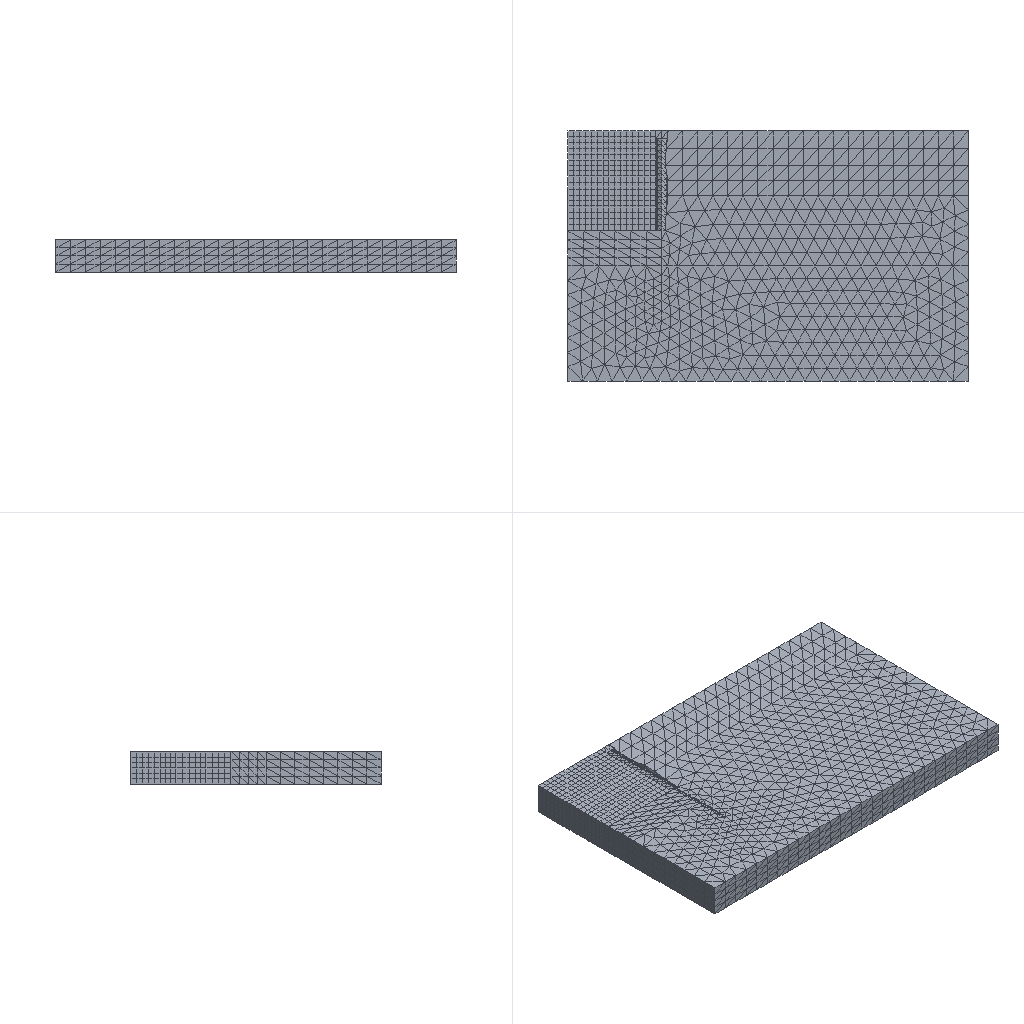Simulation study | abaqus
Set-up summary:
category,name,step,type,value,unit,region
solver,abaqus
solver,version,,,Abaqus/Standard 2020
units,not stated in the deck,,not stated
analysis,deck,,static,static
load_step,Step-delete-all,Step-delete-all,static
load_step,Step-add-zhuang,Step-add-zhuang,static
load_step,Step-geo-final,Step-geo-final,geostatic
load_step,Step-dig-lay1,Step-dig-lay1,static
load_step,Step-add-maosuo1,Step-add-maosuo1,static
load_step,Step-dig-lay2,Step-dig-lay2,static
load_step,Step-add-maosuo2,Step-add-maosuo2,static
load_step,Step-dig-lay3,Step-dig-lay3,static
load_step,requested,,,8
mesh,nodes,,,14615
mesh,elements,,,20579
element_type,C3D4,,solid,13823
element_type,T3D2,,truss,20
element_type,C3D8R,,solid,6736
load,load commands in deck,,count,9
bc,support commands in deck,,count,28
material,LAY-1,,in results
material,LAY-2,,in results
material,LAY-3,,in results
material,LAY-4,,in results
material,MAOSUO,,in results
material,STEEL,,in results
material,ZHUANG-CEMENT,,in results
material,ZHUANG-HUBI,,in results
check,setup vs results,,match,"per instance, exact: element labels, types and connectivity; labels of the nodes the elements use; coordinates of those nodes at SINGLE_PRECISION in 4 of 7 instance(s)"
Abaqus input file, long lists of numbers shortened:
*Heading
** Job name: Job-1 Model name: Model-1
** Generated by: Abaqus/CAE 2020
*Preprint, echo=NO, model=NO, history=NO, contact=NO
**
** PARTS
**
*Part, name=Part-2
*Node
      1,        -250.,      -10000.,        1850.
      2,  -355.051,      -10000.,        1600.
** (2613 more lines like these left out)
*Element, type=C3D4
   1, 1661, 1662,  800,  799
   2, 1661, 1663, 1664, 1665
** (11001 more lines like these left out)
*Nset, nset=Set-1
   47,   48,   49,   50,   51,   52,   63,   64,   65,   66,  254,  255,  256,  258,  259,  260
  261,  262,  263,  264,  265,  266,  267,  268,  269,  270,  271,  272,  273,  274,  275,  276
** (21 more lines like these left out)
*Elset, elset=Set-1, generate
  9778,  11003,      1
*Nset, nset=Set-2
   20,   21,   22,   23,   26,   27,   47,   48,   49,   50,   51,   52,   83,   87,   88,   89
   90,   91,   92,   93,   94,   95,   96,   97,   98,   99,  100,  101,  102,  103,  104,  105
** (20 more lines like these left out)
*Elset, elset=Set-2, generate
 3019,  4197,     1
*Nset, nset=Set-3
    1,    2,    3,    4,    5,    6,    7,    8,    9,   10,   11,   12,   13,   14,   15,   16
   17,   18,   19,   20,   21,   22,   23,   24,   25,   26,   27,   28,   29,   30,   31,   32
** (51 more lines like these left out)
*Elset, elset=Set-3, generate
    1,  3018,     1
*Nset, nset=Set-4
   33,   34,   35,   37,   38,   40,   41,   42,   43,   46,   53,   54,   55,   56,   57,   58
   59,   60,   61,   62,  141,  142,  143,  144,  145,  146,  147,  148,  149,  150,  151,  152
** (85 more lines like these left out)
*Elset, elset=Set-4, generate
 4198,  9777,     1
** Section: lay3
*Solid Section, elset=Set-3, material=lay-3
,
** Section: lay-2
*Solid Section, elset=Set-2, material=lay-2
,
** Section: lay4
*Solid Section, elset=Set-4, material=lay-4
,
** Section: lay1
*Solid Section, elset=Set-1, material=lay-1
,
*End Part
**
*Part, name=Part-4
*Node
      1,  -198.585,  -2785.345,   3474.874
      2,  -198.585,  -11785.345,   3474.874
** (800 more lines like these left out)
*Element, type=C3D4
  1, 313, 333, 115, 116
  2, 275,  37, 625, 258
** (2818 more lines like these left out)
*Nset, nset=Set-4
   1,   2,   5,   6,   7,   8,   9,  12,  13,  14,  15,  16,  17,  26,  28,  29
  31,  32,  33,  34,  35,  36,  37,  38,  39,  40,  41,  42,  43,  44,  45,  60
** (39 more lines like these left out)
*Elset, elset=Set-4
  630,  631,  632,  633,  634,  635,  636,  637,  638,  639,  640,  641,  642,  643,  644,  645
  646,  647,  648,  649,  650,  651,  652,  653,  654,  655,  656,  657,  658,  659,  660,  661
** (127 more lines like these left out)
*Nset, nset=Set-5
   1,   2,   3,   4,   5,   6,   7,   8,   9,  10,  11,  12,  34,  35,  36,  37
  38,  39,  40,  41,  42,  43,  44,  45,  46,  47,  48,  49,  50,  51,  52,  53
** (11 more lines like these left out)
*Elset, elset=Set-5, generate
   1,  629,    1
*Nset, nset=Set-6
  13,  14,  15,  18,  19,  20,  21,  22,  23,  24,  25,  26,  27,  28,  29,  30
 118, 119, 120, 121, 122, 183, 184, 185, 186, 187, 188, 189, 190, 191, 192, 193
** (2 more lines like these left out)
*Elset, elset=Set-6, generate
 1645,  1779,     1
** Section: zhuang-cement
*Solid Section, elset=Set-5, material=zhuang-cement
,
** Section: zhuang-hubi
*Solid Section, elset=Set-4, material=zhuang-hubi
,
** Section: zhuang-hubi
*Solid Section, elset=Set-6, material=zhuang-hubi
,
*End Part
**
*Part, name=digit
*Node
      1,        8800.,       -7500.,           0.
      2,        8800.,       -7500.,        3200.
** (2014 more lines like these left out)
*Element, type=C3D8R
  1,   84,  415, 1177,  331,    1,   25,  301,   40
  2,  415,  416, 1178, 1177,   25,   26,  302,  301
** (1528 more lines like these left out)
*Nset, nset=Set-1
   11,   12,   14,   15,   21,   22,   23,   24,  119,  120,  121,  122,  123,  131,  132,  133
  134,  135,  137,  138,  139,  140,  141,  142,  143,  144,  145,  146,  147,  148,  149,  150
** (47 more lines like these left out)
*Elset, elset=Set-1, generate
  991,  1530,     1
*Nset, nset=Set-2
    9,   10,   11,   12,   13,   14,   15,   16,   17,   18,   19,   20,  113,  114,  115,  116
  117,  118,  119,  120,  121,  122,  123,  124,  125,  126,  127,  128,  129,  130,  131,  132
** (40 more lines like these left out)
*Elset, elset=Set-2
 361, 362, 363, 364, 365, 366, 367, 368, 369, 370, 371, 372, 373, 374, 375, 376
 377, 378, 379, 380, 381, 382, 383, 384, 385, 386, 387, 388, 389, 390, 391, 392
** (27 more lines like these left out)
*Nset, nset=Set-3
    1,    2,    3,    4,    5,    6,    7,    8,   17,   18,   19,   20,   25,   26,   27,   28
   29,   30,   31,   32,   33,   34,   35,   36,   37,   38,   39,   40,   41,   42,   43,   44
** (47 more lines like these left out)
*Elset, elset=Set-3
   1,   2,   3,   4,   5,   6,   7,   8,   9,  10,  11,  12,  13,  14,  15,  16
  17,  18,  19,  20,  21,  22,  23,  24,  25,  26,  27,  28,  29,  30,  31,  32
** (32 more lines like these left out)
*Nset, nset=dig
    9,   10,   11,   12,   13,   14,   15,   16,   21,   22,   23,   24,  113,  114,  115,  116
  117,  118,  119,  120,  121,  122,  123,  124,  125,  126,  127,  128,  129,  130,  131,  132
** (61 more lines like these left out)
*Elset, elset=dig
  361,  362,  363,  364,  365,  366,  367,  368,  369,  370,  371,  372,  373,  374,  375,  376
  377,  378,  379,  380,  381,  382,  383,  384,  385,  386,  387,  388,  389,  390,  391,  392
** (43 more lines like these left out)
*Nset, nset=dig2
    1,    2,    5,    8,    9,   10,   13,   16,   17,   18,   19,   20,   25,   26,   27,   28
   29,   41,   42,   43,   44,   45,   71,   72,   73,   74,   75,   76,   77,   78,   79,   80
** (40 more lines like these left out)
*Elset, elset=dig2, generate
 541,  990,    1
*Nset, nset=dig3
    1,    2,    3,    4,    5,    6,    7,    8,   25,   26,   27,   28,   29,   30,   31,   32
   33,   34,   35,   36,   37,   38,   39,   40,   41,   42,   43,   44,   45,   46,   47,   48
** (33 more lines like these left out)
*Elset, elset=dig3, generate
   1,  360,    1
*Nset, nset=Set-9
    9,   10,   11,   12,   13,   14,   15,   16,   21,   22,   23,   24,  113,  114,  115,  116
  117,  118,  119,  120,  121,  122,  123,  124,  125,  126,  127,  128,  129,  130,  131,  132
** (61 more lines like these left out)
*Elset, elset=Set-9
  361,  362,  363,  364,  365,  366,  367,  368,  369,  370,  371,  372,  373,  374,  375,  376
  377,  378,  379,  380,  381,  382,  383,  384,  385,  386,  387,  388,  389,  390,  391,  392
** (43 more lines like these left out)
*Nset, nset=Set-10
    1,    2,    5,    8,    9,   10,   13,   16,   17,   18,   19,   20,   25,   26,   27,   28
   29,   41,   42,   43,   44,   45,   71,   72,   73,   74,   75,   76,   77,   78,   79,   80
** (40 more lines like these left out)
*Elset, elset=Set-10, generate
 541,  990,    1
*Nset, nset=Set-11
    1,    2,    3,    4,    5,    6,    7,    8,   25,   26,   27,   28,   29,   30,   31,   32
   33,   34,   35,   36,   37,   38,   39,   40,   41,   42,   43,   44,   45,   46,   47,   48
** (33 more lines like these left out)
*Elset, elset=Set-11, generate
   1,  360,    1
*Nset, nset=Set-12
   11,   12,   14,   15,   21,   22,   23,   24,  119,  120,  121,  122,  123,  131,  132,  133
  134,  135,  137,  138,  139,  140,  141,  142,  143,  144,  145,  146,  147,  148,  149,  150
** (47 more lines like these left out)
*Elset, elset=Set-12, generate
  991,  1530,     1
*Nset, nset=Set-13
    9,   10,   11,   12,   13,   14,   15,   16,   17,   18,   19,   20,  113,  114,  115,  116
  117,  118,  119,  120,  121,  122,  123,  124,  125,  126,  127,  128,  129,  130,  131,  132
** (40 more lines like these left out)
*Elset, elset=Set-13
 361, 362, 363, 364, 365, 366, 367, 368, 369, 370, 371, 372, 373, 374, 375, 376
 377, 378, 379, 380, 381, 382, 383, 384, 385, 386, 387, 388, 389, 390, 391, 392
** (27 more lines like these left out)
*Nset, nset=Set-14
    1,    2,    3,    4,    5,    6,    7,    8,   17,   18,   19,   20,   25,   26,   27,   28
   29,   30,   31,   32,   33,   34,   35,   36,   37,   38,   39,   40,   41,   42,   43,   44
** (47 more lines like these left out)
*Elset, elset=Set-14
   1,   2,   3,   4,   5,   6,   7,   8,   9,  10,  11,  12,  13,  14,  15,  16
  17,  18,  19,  20,  21,  22,  23,  24,  25,  26,  27,  28,  29,  30,  31,  32
** (32 more lines like these left out)
** Section: lay3
*Solid Section, elset=Set-14, material=lay-3
,
** Section: lay-2
*Solid Section, elset=Set-13, material=lay-2
,
** Section: lay1
*Solid Section, elset=Set-12, material=lay-1
,
*End Part
**
*Part, name=maosuo-d27
*Node
      1,           0.,           0.,           0.
      2,   1556.389,  -1089.795,           0.
** (9 more lines like these left out)
*Element, type=T3D2
 1,  1,  2
 2,  2,  3
** (8 more lines like these left out)
*Nset, nset=Set-1, generate
  1,  11,   1
*Elset, elset=Set-1, generate
  1,  10,   1
** Section: maosuo-d27
*Solid Section, elset=Set-1, material=maosuo
572.,
*End Part
**
*Part, name=maosuo-d33
*Node
      1,           0.,           0.,           0.
      2,   1884.05,  -1319.226,           0.
** (9 more lines like these left out)
*Element, type=T3D2
 1,  1,  2
 2,  2,  3
** (8 more lines like these left out)
*Nset, nset=Set-1, generate
  1,  11,   1
*Elset, elset=Set-1, generate
  1,  10,   1
** Section: mosuo-d33
*Solid Section, elset=Set-1, material=maosuo
855.,
*End Part
**
*Part, name=work-5
*Node
      1,  -345.475,   11544.227,        3350.
      2,  -45.475,   11544.227,        3350.
** (4578 more lines like these left out)
*Element, type=C3D8R
  1,  239,  240, 1295, 1296,  339,  340, 1342, 1343
  2,  166, 1280, 1279,  165,  266, 1327, 1326,  265
** (2601 more lines like these left out)
*Nset, nset=Set-2, generate
    1,  4580,     1
*Elset, elset=Set-2, generate
    1,  2603,     1
*Nset, nset=work5-insert-down
   25,   26,   27,   28,   29,   30,   31,   32,   33,   34,   35,   36,   37,   38,   39,   40
   41,   42,   43,   44,   45,   46,   47,   48,   49,   50,   51,   52,   53,   54,   55,   56
** (172 more lines like these left out)
*Elset, elset=work5-insert-down, generate
  686,  2603,     1
*Nset, nset=w5-insert-up
    1,    2,    3,    4,    5,    6,    7,    8,    9,   10,   11,   12,   13,   14,   15,   16
   17,   18,   19,   20,   21,   22,   23,   24,   73,   74,   75,   76,   77,   78,   79,   80
** (24 more lines like these left out)
*Elset, elset=w5-insert-up, generate
   1,  137,    1
** Section: steel
*Solid Section, elset=Set-2, material=steel
,
*End Part
**
**
** ASSEMBLY
**
*Assembly, name=Assembly
**
*Instance, name=Part-2-1, part=Part-2
*End Instance
**
*Instance, name=work-5-2, part=work-5
       2600.,  -155.773,  1654.525
       2600.,  -155.773,  1654.525, 2600.707,  -155.773, 1653.818,         180.
*End Instance
**
*Instance, name=digit-1, part=digit
     -10000.,           0.,           0.
*End Instance
**
*Instance, name=Part-4-1, part=Part-4
      -3800.,  -714.655,  1868.082
      -3800.,  -714.655,  1868.082,       -3800., -713.655,  1868.082, 90.
*End Instance
**
*Instance, name=maosuo-d27-1, part=maosuo-d27
          0.,       -7000.,        2600.
*End Instance
**
*Instance, name=maosuo-d33-1, part=maosuo-d33
          0.,       -4000.,         600.
*End Instance
**
*Instance, name=work-5-1, part=work-5
      -3800., -155.773,  1545.475
      -3800., -155.773,  1545.475, -3799.293, -155.773, 1546.182,         180.
*End Instance
**
*Nset, nset=Set-3, instance=maosuo-d27-1, generate
  1,  11,   1
*Nset, nset=Set-3, instance=maosuo-d33-1, generate
  1,  11,   1
*Elset, elset=Set-3, instance=maosuo-d27-1, generate
  1,  10,   1
*Elset, elset=Set-3, instance=maosuo-d33-1, generate
  1,  10,   1
*Nset, nset=Set-4, instance=maosuo-d27-1, generate
  1,  11,   1
*Nset, nset=Set-4, instance=maosuo-d33-1, generate
  1,  11,   1
*Elset, elset=Set-4, instance=maosuo-d27-1, generate
  1,  10,   1
*Elset, elset=Set-4, instance=maosuo-d33-1, generate
  1,  10,   1
*Nset, nset=Set-7, instance=Part-2-1
   59,   60,   61,   62,  334,  335,  336,  351,  352,  353,  354,  355,  356,  357,  358,  359
  360,  361,  362,  363,  364,  365,  366,  367,  368,  369,  370,  371,  372,  373,  374,  375
** (7 more lines like these left out)
*Elset, elset=Set-7, instance=Part-2-1
 4241, 4282, 4399, 4468, 4559, 4637, 4778, 5047, 5050, 5090, 5092, 5094, 5098, 5100, 5213, 5425
 5574, 5599, 5677, 5757, 5792, 5802, 5857, 5866, 5912, 5920, 5933, 5943, 5945, 5948, 5957, 6032
** (12 more lines like these left out)
*Nset, nset=Set-8, instance=Part-2-1
   26,   27,   34,   42,   43,   44,   45,   46,   47,   48,   59,   60,   61,   62,   63,   64
  106,  107,  108,  161,  162,  163,  164,  194,  195,  196,  197,  218,  219,  220,  226,  227
** (8 more lines like these left out)
*Elset, elset=Set-8, instance=Part-2-1
    65,    70,    86,    87,    88,   132,   137,   260,   350,   395,   401,   458,   474,   475,   566,   653
   880,  1001,  1120,  1123,  1180,  1181,  1210,  1329,  1339,  1509,  1510,  1511,  1515,  1567,  1571,  1628
** (13 more lines like these left out)
*Nset, nset=Set-9, instance=Part-2-1
    8,    9,   20,   23,   24,   25,   26,   27,   33,   34,   38,   42,   43,   44,   45,   46
   47,   48,   49,   50,   53,   58,   59,   60,   61,   62,   63,   64,   65,   66,   84,   85
** (64 more lines like these left out)
*Elset, elset=Set-9, instance=Part-2-1
    11,    16,    25,    49,    53,    58,    63,    67,    86,    89,   105,   107,   160,   162,   173,   186
   196,   210,   235,   241,   245,   248,   275,   280,   282,   295,   297,   324,   327,   335,   369,   382
** (118 more lines like these left out)
*Nset, nset=Set-15, instance=work-5-2, generate
    1,  4580,     1
*Nset, nset=Set-15, instance=Part-4-1, generate
   1,  802,    1
*Nset, nset=Set-15, instance=maosuo-d27-1, generate
  1,  11,   1
*Nset, nset=Set-15, instance=maosuo-d33-1, generate
  1,  11,   1
*Nset, nset=Set-15, instance=work-5-1, generate
    1,  4580,     1
*Elset, elset=Set-15, instance=work-5-2, generate
    1,  2603,     1
*Elset, elset=Set-15, instance=Part-4-1, generate
    1,  2820,     1
*Elset, elset=Set-15, instance=maosuo-d27-1, generate
  1,  10,   1
*Elset, elset=Set-15, instance=maosuo-d33-1, generate
  1,  10,   1
*Elset, elset=Set-15, instance=work-5-1, generate
    1,  2603,     1
*Nset, nset=Set-16, instance=Part-2-1, generate
    1,  2615,     1
*Elset, elset=Set-16, instance=Part-2-1, generate
     1,  11003,      1
*Nset, nset=Set-17, instance=work-5-2, generate
    1,  4580,     1
*Nset, nset=Set-17, instance=Part-4-1, generate
   1,  802,    1
*Nset, nset=Set-17, instance=work-5-1, generate
    1,  4580,     1
*Elset, elset=Set-17, instance=work-5-2, generate
    1,  2603,     1
*Elset, elset=Set-17, instance=Part-4-1, generate
    1,  2820,     1
*Elset, elset=Set-17, instance=work-5-1, generate
    1,  2603,     1
*Nset, nset=Set-18, instance=work-5-2, generate
    1,  4580,     1
*Nset, nset=Set-18, instance=Part-4-1, generate
   1,  802,    1
*Nset, nset=Set-18, instance=work-5-1, generate
    1,  4580,     1
*Elset, elset=Set-18, instance=work-5-2, generate
    1,  2603,     1
*Elset, elset=Set-18, instance=Part-4-1, generate
    1,  2820,     1
*Elset, elset=Set-18, instance=work-5-1, generate
    1,  2603,     1
*Nset, nset=Set-19, instance=maosuo-d33-1, generate
  1,  11,   1
*Elset, elset=Set-19, instance=maosuo-d33-1, generate
  1,  10,   1
*Nset, nset=Set-20, instance=maosuo-d27-1, generate
  1,  11,   1
*Nset, nset=Set-20, instance=maosuo-d33-1, generate
  1,  11,   1
*Elset, elset=Set-20, instance=maosuo-d27-1, generate
  1,  10,   1
*Elset, elset=Set-20, instance=maosuo-d33-1, generate
  1,  10,   1
*Nset, nset=Set-21, instance=maosuo-d33-1, generate
  1,  11,   1
*Elset, elset=Set-21, instance=maosuo-d33-1, generate
  1,  10,   1
*Nset, nset=Set-22, instance=maosuo-d33-1, generate
  1,  11,   1
*Elset, elset=Set-22, instance=maosuo-d33-1, generate
  1,  10,   1
*Nset, nset=Set-23, instance=maosuo-d27-1, generate
  1,  11,   1
*Elset, elset=Set-23, instance=maosuo-d27-1, generate
  1,  10,   1
*Nset, nset=Set-24, instance=maosuo-d27-1, generate
  1,  11,   1
*Elset, elset=Set-24, instance=maosuo-d27-1, generate
  1,  10,   1
*Nset, nset=Set-25, instance=maosuo-d27-1, generate
  1,  11,   1
*Elset, elset=Set-25, instance=maosuo-d27-1, generate
  1,  10,   1
*Nset, nset=Set-26, instance=Part-2-1
   26,   27,   34,   42,   43,   44,   45,   46,   47,   48,   59,   60,   61,   62,   63,   64
  106,  107,  108,  161,  162,  163,  164,  194,  195,  196,  197,  218,  219,  220,  226,  227
** (8 more lines like these left out)
*Nset, nset=Set-26, instance=digit-1
    5,    6,    7,    8,   13,   14,   15,   16,   19,   20,   21,   24,   41,   42,   43,   44
   45,   46,   47,   48,   49,   50,   51,   52,   53,   54,   55,   56,  125,  126,  127,  128
** (6 more lines like these left out)
*Elset, elset=Set-26, instance=Part-2-1
    65,    70,    86,    87,    88,   132,   137,   260,   350,   395,   401,   458,   474,   475,   566,   653
   880,  1001,  1120,  1123,  1180,  1181,  1210,  1329,  1339,  1509,  1510,  1511,  1515,  1567,  1571,  1628
** (13 more lines like these left out)
*Elset, elset=Set-26, instance=digit-1
  337,  338,  339,  340,  341,  342,  343,  344,  345,  346,  347,  348,  349,  350,  351,  352
  353,  354,  355,  356,  357,  358,  359,  360,  529,  530,  531,  532,  533,  534,  535,  536
** (5 more lines like these left out)
*Nset, nset=Set-27, instance=Part-2-1
    8,    9,   20,   23,   24,   25,   26,   27,   33,   34,   38,   42,   43,   44,   45,   46
   47,   48,   49,   50,   53,   58,   59,   60,   61,   62,   63,   64,   65,   66,   84,   85
** (64 more lines like these left out)
*Nset, nset=Set-27, instance=digit-1
    1,    2,    3,    4,    5,    6,    7,    8,    9,   10,   11,   12,   13,   14,   15,   16
   17,   18,   19,   20,   21,   22,   23,   24,   30,   31,   32,   38,   39,   40,   46,   47
** (34 more lines like these left out)
*Elset, elset=Set-27, instance=Part-2-1
    11,    16,    25,    49,    53,    58,    63,    67,    86,    89,   105,   107,   160,   162,   173,   186
   196,   210,   235,   241,   245,   248,   275,   280,   282,   295,   297,   324,   327,   335,   369,   382
** (118 more lines like these left out)
*Elset, elset=Set-27, instance=digit-1
    1,    6,    7,   12,   13,   18,   19,   24,   25,   30,   31,   36,   37,   42,   43,   48
   49,   54,   55,   60,   61,   66,   67,   72,   73,   78,   79,   84,   85,   90,   91,   96
** (30 more lines like these left out)
*Nset, nset=Set-28, instance=Part-2-1
   26,   27,   34,   42,   43,   44,   45,   46,   47,   48,   59,   60,   61,   62,   63,   64
  106,  107,  108,  161,  162,  163,  164,  194,  195,  196,  197,  218,  219,  220,  226,  227
** (8 more lines like these left out)
*Elset, elset=Set-28, instance=Part-2-1
    65,    70,    86,    87,    88,   132,   137,   260,   350,   395,   401,   458,   474,   475,   566,   653
   880,  1001,  1120,  1123,  1180,  1181,  1210,  1329,  1339,  1509,  1510,  1511,  1515,  1567,  1571,  1628
** (13 more lines like these left out)
*Nset, nset=Set-29, instance=Part-2-1
    7,    9,   19,   20,   21,   22,   23,   24,   49,   50,   51,   52,   65,   66,   81,   83
   84,   85,  277,  278,  298,  418,  457,  458,  459,  460,  464,  465,  466,  467,  468,  469
** (1 more lines like these left out)
*Nset, nset=Set-29, instance=digit-1
    1,    2,    3,    4,    5,    6,    7,    8,    9,   10,   11,   12,   13,   14,   15,   16
   17,   18,   19,   20,   21,   22,   23,   24,   25,   26,   27,   28,   29,   30,   31,   32
** (14 more lines like these left out)
*Elset, elset=Set-29, instance=Part-2-1
    63,  1322,  1376,  1630,  1676,  1809,  1928,  1940,  1945,  1952,  1956,  1960,  1966,  1967,  1971,  1973
  1976,  1990,  1991,  2000,  2001,  2010,  2011,  2039,  2044,  2051,  2054,  2077,  3020,  3022,  3032,  3113
** (3 more lines like these left out)
*Elset, elset=Set-29, instance=digit-1
    1,    2,    3,    4,    5,    6,    7,    8,    9,   10,   11,   12,   13,   14,   15,   16
   17,   18,   19,   20,   21,   22,   23,   24,  337,  338,  339,  340,  341,  342,  343,  344
** (11 more lines like these left out)
*Nset, nset=Set-30, instance=Part-2-1
   26,   27,   34,   42,   43,   44,   45,   46,   47,   48,   59,   60,   61,   62,   63,   64
  106,  107,  108,  161,  162,  163,  164,  194,  195,  196,  197,  218,  219,  220,  226,  227
** (8 more lines like these left out)
*Nset, nset=Set-30, instance=digit-1
    5,    6,    7,    8,   13,   14,   15,   16,   19,   20,   21,   24,   41,   42,   43,   44
   45,   46,   47,   48,   49,   50,   51,   52,   53,   54,   55,   56,  125,  126,  127,  128
** (6 more lines like these left out)
*Elset, elset=Set-30, instance=Part-2-1
    65,    70,    86,    87,    88,   132,   137,   260,   350,   395,   401,   458,   474,   475,   566,   653
   880,  1001,  1120,  1123,  1180,  1181,  1210,  1329,  1339,  1509,  1510,  1511,  1515,  1567,  1571,  1628
** (13 more lines like these left out)
*Elset, elset=Set-30, instance=digit-1
  337,  338,  339,  340,  341,  342,  343,  344,  345,  346,  347,  348,  349,  350,  351,  352
  353,  354,  355,  356,  357,  358,  359,  360,  529,  530,  531,  532,  533,  534,  535,  536
** (5 more lines like these left out)
*Nset, nset=Set-31, instance=Part-2-1
    7,    9,   19,   20,   21,   22,   23,   24,   49,   50,   51,   52,   65,   66,   81,   83
   84,   85,  277,  278,  298,  418,  457,  458,  459,  460,  464,  465,  466,  467,  468,  469
** (1 more lines like these left out)
*Nset, nset=Set-31, instance=digit-1
    1,    2,    3,    4,    9,   10,   11,   12,   17,   18,   22,   23,   25,   26,   27,   28
   29,   30,   31,   32,   33,   34,   35,   36,   37,   38,   39,   40,  113,  114,  115,  116
** (6 more lines like these left out)
*Elset, elset=Set-31, instance=Part-2-1
    63,  1322,  1376,  1630,  1676,  1809,  1928,  1940,  1945,  1952,  1956,  1960,  1966,  1967,  1971,  1973
  1976,  1990,  1991,  2000,  2001,  2010,  2011,  2039,  2044,  2051,  2054,  2077,  3020,  3022,  3032,  3113
** (3 more lines like these left out)
*Elset, elset=Set-31, instance=digit-1
    1,    2,    3,    4,    5,    6,    7,    8,    9,   10,   11,   12,   13,   14,   15,   16
   17,   18,   19,   20,   21,   22,   23,   24,  361,  362,  363,  364,  365,  366,  367,  368
** (5 more lines like these left out)
*Nset, nset=Set-32, instance=Part-4-1
 15, 18, 19, 20, 21, 22, 23, 24, 25, 27, 29, 30
*Elset, elset=Set-32, instance=Part-4-1
 1667, 1668, 1680, 1690, 1697, 1708, 1715, 1743
*Nset, nset=Set-33, instance=Part-2-1
   26,   27,   34,   42,   43,   44,   45,   46,   47,   48,   59,   60,   61,   62,   63,   64
  106,  107,  108,  161,  162,  163,  164,  194,  195,  196,  197,  218,  219,  220,  226,  227
** (8 more lines like these left out)
*Elset, elset=Set-33, instance=Part-2-1
    65,    70,    86,    87,    88,   132,   137,   260,   350,   395,   401,   458,   474,   475,   566,   653
   880,  1001,  1120,  1123,  1180,  1181,  1210,  1329,  1339,  1509,  1510,  1511,  1515,  1567,  1571,  1628
** (13 more lines like these left out)
*Nset, nset=Set-34, instance=Part-2-1
   26,   27,   34,   42,   43,   44,   45,   46,   47,   48,   59,   60,   61,   62,   63,   64
  106,  107,  108,  161,  162,  163,  164,  194,  195,  196,  197,  218,  219,  220,  226,  227
** (8 more lines like these left out)
*Elset, elset=Set-34, instance=Part-2-1
    65,    70,    86,    87,    88,   132,   137,   260,   350,   395,   401,   458,   474,   475,   566,   653
   880,  1001,  1120,  1123,  1180,  1181,  1210,  1329,  1339,  1509,  1510,  1511,  1515,  1567,  1571,  1628
** (13 more lines like these left out)
*Nset, nset=Set-35, instance=digit-1
   13,   14,   15,   16,   21,   24,  125,  126,  127,  128,  129,  130,  131,  132,  133,  134
  135,  136,  276,  277,  278,  279,  280,  281,  282,  283,  284,  285,  286,  287,  288,  289
** (2 more lines like these left out)
*Elset, elset=Set-35, instance=digit-1
  529,  530,  531,  532,  533,  534,  535,  536,  537,  538,  539,  540,  991, 1006, 1021, 1036
 1051, 1066, 1081, 1096, 1111, 1126, 1141, 1156, 1171, 1186, 1201, 1216, 1231, 1246, 1261, 1276
** (1 more lines like these left out)
*Nset, nset=Set-36, instance=digit-1
   5,   8,  13,  16,  19,  20,  41,  42,  43,  44,  45, 125, 126, 127, 128, 129
 200, 201, 202, 203, 204, 205, 206, 239, 240, 241, 242, 738, 739, 740, 741, 742
** (1 more lines like these left out)
*Elset, elset=Set-36, instance=digit-1
 709, 710, 711, 712, 713, 714, 715, 716, 717, 718, 719, 720, 973, 974, 975, 976
 977, 978, 979, 980, 981, 982, 983, 984, 985, 986, 987, 988, 989, 990
*Nset, nset=Set-37, instance=digit-1
   5,   6,   7,   8,  41,  42,  43,  44,  45,  46,  47,  48,  49,  50,  51,  52
  53,  54,  55,  56, 316, 317, 318, 319, 320, 321, 322, 323, 324, 325, 326, 327
** (1 more lines like these left out)
*Elset, elset=Set-37, instance=digit-1, generate
 337,  360,    1
*Nset, nset=Set-38, instance=Part-2-1
    8,    9,   20,   23,   24,   25,   26,   27,   33,   34,   38,   42,   43,   44,   45,   46
   47,   48,   49,   50,   53,   58,   59,   60,   61,   62,   63,   64,   65,   66,   84,   85
** (64 more lines like these left out)
*Elset, elset=Set-38, instance=Part-2-1
    11,    16,    25,    49,    53,    58,    63,    67,    86,    89,   105,   107,   160,   162,   173,   186
   196,   210,   235,   241,   245,   248,   275,   280,   282,   295,   297,   324,   327,   335,   369,   382
** (118 more lines like these left out)
*Nset, nset=Set-39, instance=digit-1
    9,   10,   11,   12,   13,   14,   15,   16,   21,   22,   23,   24,  118,  124,  130,  136
  137,  138,  139,  140,  141,  142,  143,  144,  145,  146,  147,  148,  149,  150,  151,  152
** (16 more lines like these left out)
*Elset, elset=Set-39, instance=digit-1
  361,  366,  367,  372,  373,  378,  379,  384,  385,  390,  391,  396,  397,  402,  403,  408
  409,  414,  415,  420,  421,  426,  427,  432,  433,  438,  439,  444,  445,  450,  451,  456
** (13 more lines like these left out)
*Nset, nset=Set-40, instance=digit-1
   1,   2,   5,   8,   9,  10,  13,  16,  17,  18,  19,  20,  71,  72,  73,  74
  75,  76,  77,  78,  79,  80,  81,  82,  83,  84,  99, 100, 101, 102, 103, 104
** (10 more lines like these left out)
*Elset, elset=Set-40, instance=digit-1
 541, 546, 547, 552, 553, 558, 559, 564, 565, 570, 571, 576, 577, 582, 583, 588
 589, 594, 595, 600, 601, 606, 607, 612, 613, 618, 619, 624, 625, 630, 631, 636
** (8 more lines like these left out)
*Nset, nset=Set-41, instance=digit-1
   1,   2,   3,   4,   5,   6,   7,   8,  30,  31,  32,  38,  39,  40,  46,  47
  48,  54,  55,  56,  57,  58,  59,  60,  61,  62,  63,  64,  65,  66,  67,  68
** (8 more lines like these left out)
*Elset, elset=Set-41, instance=digit-1
   1,   6,   7,  12,  13,  18,  19,  24,  25,  30,  31,  36,  37,  42,  43,  48
  49,  54,  55,  60,  61,  66,  67,  72,  73,  78,  79,  84,  85,  90,  91,  96
** (6 more lines like these left out)
*Nset, nset=m_Set-1, instance=work-5-2
   49,   50,   51,   52,   53,   54,   55,   56,   57,   58,   59,   60,   61,   62,   63,   64
   65,   66,   67,   68,   69,   70,   71,   72,  921,  922,  923,  924,  925,  926,  927,  928
** (27 more lines like these left out)
*Elset, elset=m_Set-1, instance=work-5-2, generate
 2467,  2603,     1
*Nset, nset=m_Set-5, instance=maosuo-d27-1, generate
  1,  11,   1
*Nset, nset=m_Set-5, instance=maosuo-d33-1, generate
  1,  11,   1
*Elset, elset=m_Set-5, instance=maosuo-d27-1, generate
  1,  10,   1
*Elset, elset=m_Set-5, instance=maosuo-d33-1, generate
  1,  10,   1
*Nset, nset=m_Set-11, instance=work-5-2
   49,   50,   51,   52,   53,   54,   55,   56,   57,   58,   59,   60,   61,   62,   63,   64
   65,   66,   67,   68,   69,   70,   71,   72,  921,  922,  923,  924,  925,  926,  927,  928
** (27 more lines like these left out)
*Nset, nset=m_Set-11, instance=work-5-1
   49,   50,   51,   52,   53,   54,   55,   56,   57,   58,   59,   60,   61,   62,   63,   64
   65,   66,   67,   68,   69,   70,   71,   72,  921,  922,  923,  924,  925,  926,  927,  928
** (27 more lines like these left out)
*Elset, elset=m_Set-11, instance=work-5-2, generate
 2467,  2603,     1
*Elset, elset=m_Set-11, instance=work-5-1, generate
 2467,  2603,     1
*Nset, nset=m_Set-13, instance=work-5-2
    1,    2,    3,    4,    5,    6,    7,    8,    9,   10,   11,   12,   13,   14,   15,   16
   17,   18,   19,   20,   21,   22,   23,   24,   25,   26,   27,   28,   29,   30,   31,   32
** (213 more lines like these left out)
*Nset, nset=m_Set-13, instance=work-5-1
    1,    2,    3,    4,    5,    6,    7,    8,    9,   10,   11,   12,   13,   14,   15,   16
   17,   18,   19,   20,   21,   22,   23,   24,   25,   26,   27,   28,   29,   30,   31,   32
** (213 more lines like these left out)
*Elset, elset=m_Set-13, instance=work-5-2, generate
    1,  1918,     1
*Elset, elset=m_Set-13, instance=work-5-1, generate
    1,  1918,     1
*Nset, nset=s_Set-5, instance=Part-2-1, generate
    1,  2615,     1
*Elset, elset=s_Set-5, instance=Part-2-1, generate
     1,  11003,      1
*Nset, nset=s_Set-10, instance=Part-4-1
   1,   2,   5,   6,   7,   8,   9,  12,  13,  14,  15,  16,  17,  18,  19,  20
  21,  22,  23,  24,  25,  26,  27,  28,  29,  30,  31,  32,  33,  34,  35,  36
** (41 more lines like these left out)
*Elset, elset=s_Set-10, instance=Part-4-1, generate
  630,  2820,     1
*Nset, nset=s_Set-11, instance=Part-4-1
  13,  14,  15,  18,  19,  20,  21,  22,  23,  24,  25,  26,  27,  28,  29,  30
 118, 119, 120, 121, 122, 183, 184, 185, 186, 187, 188, 189, 190, 191, 192, 193
** (2 more lines like these left out)
*Elset, elset=s_Set-11, instance=Part-4-1, generate
 1645,  1779,     1
*Nset, nset=s_Set-13, instance=Part-4-1
   1,   2,   3,   4,   5,   6,   7,   8,   9,  10,  11,  12,  34,  35,  36,  37
  38,  39,  40,  41,  42,  43,  44,  45,  46,  47,  48,  49,  50,  51,  52,  53
** (11 more lines like these left out)
*Elset, elset=s_Set-13, instance=Part-4-1, generate
   1,  629,    1
*Elset, elset=_m_Surf-1_END1, internal, instance=maosuo-d27-1
 1,
*Elset, elset=_m_Surf-1_END1, internal, instance=maosuo-d33-1
 1,
*Surface, type=ELEMENT, name=m_Surf-1
_m_Surf-1_END1, END1
*Elset, elset=_m_Surf-3_S1, internal, instance=Part-4-1
    8,   69,   81,   90,  122,  132,  169,  187,  194,  234,  237,  380,  421,  455,  545,  584
  598,  599,  620,  633,  687,  870,  941,  948,  970, 1004, 1063, 1105, 1131, 1245, 1253, 1263
** (3 more lines like these left out)
*Elset, elset=_m_Surf-3_S4, internal, instance=Part-4-1
   16,   19,   23,   50,   70,   83,  107,  111,  146,  156,  160,  172,  174,  215,  235,  263
  275,  293,  294,  297,  298,  299,  314,  315,  360,  378,  386,  398,  400,  404,  411,  418
** (4 more lines like these left out)
*Elset, elset=_m_Surf-3_S2, internal, instance=Part-4-1
   47,  124,  190,  300,  340,  365,  407,  450,  528,  543,  559,  589,  601,  613,  806,  869
  878,  944,  983, 1004, 1013, 1021, 1027, 1036, 1081, 1088, 1121, 1124, 1126, 1129, 1211, 1331
** (2 more lines like these left out)
*Elset, elset=_m_Surf-3_S3, internal, instance=Part-4-1
    1,   28,   34,   40,   41,   46,   49,   57,   59,   66,   71,   75,   78,   88,  100,  101
  102,  110,  113,  117,  118,  121,  128,  129,  130,  131,  134,  135,  142,  143,  145,  148
** (54 more lines like these left out)
*Surface, type=ELEMENT, name=m_Surf-3
_m_Surf-3_S1, S1
_m_Surf-3_S4, S4
_m_Surf-3_S2, S2
_m_Surf-3_S3, S3
*Elset, elset=_m_Surf-5_S5, internal, instance=digit-1
  19,  20,  21,  22,  23,  24,  43,  44,  45,  46,  47,  48,  67,  68,  69,  70
  71,  72,  91,  92,  93,  94,  95,  96, 115, 116, 117, 118, 119, 120, 139, 140
** (4 more lines like these left out)
*Surface, type=ELEMENT, name=m_Surf-5
_m_Surf-5_S5, S5
*Elset, elset=_m_Surf-7_S1, internal, instance=Part-4-1
    8,   69,   81,   90,  122,  132,  169,  187,  194,  234,  237,  380,  421,  455,  545,  584
  598,  599,  620,  633,  687,  870,  941,  948,  970, 1004, 1063, 1105, 1131, 1245, 1253, 1263
** (3 more lines like these left out)
*Elset, elset=_m_Surf-7_S4, internal, instance=Part-4-1
   16,   19,   23,   50,   70,   83,  107,  111,  146,  156,  160,  172,  174,  202,  215,  235
  263,  275,  293,  294,  297,  298,  299,  314,  315,  360,  378,  386,  398,  400,  404,  411
** (5 more lines like these left out)
*Elset, elset=_m_Surf-7_S2, internal, instance=Part-4-1
   47,  124,  190,  300,  340,  365,  406,  407,  450,  528,  543,  559,  589,  601,  613,  806
  869,  878,  944,  983, 1004, 1013, 1021, 1027, 1036, 1081, 1088, 1121, 1124, 1126, 1129, 1211
** (3 more lines like these left out)
*Elset, elset=_m_Surf-7_S3, internal, instance=Part-4-1
    1,   13,   28,   34,   40,   41,   46,   49,   57,   59,   66,   71,   75,   78,   88,  100
  101,  102,  103,  106,  109,  110,  113,  117,  118,  121,  128,  129,  130,  131,  134,  135
** (57 more lines like these left out)
*Surface, type=ELEMENT, name=m_Surf-7
_m_Surf-7_S1, S1
_m_Surf-7_S4, S4
_m_Surf-7_S2, S2
_m_Surf-7_S3, S3
*Elset, elset=_m_Surf-9_S5, internal, instance=work-5-2
    7,    8,   12,   13,   16,   17,   18,   20,   22,   25,   26,   45,   50,   53,   54,   57
   60,   62,   64,   66,   68,   69,   83,   84,   87,   91,   92,   96,  107,  140,  141,  143
** (72 more lines like these left out)
*Elset, elset=_m_Surf-9_S5, internal, instance=work-5-1
    7,    8,   12,   13,   16,   17,   18,   20,   22,   25,   26,   45,   50,   53,   54,   57
   60,   62,   64,   66,   68,   69,   83,   84,   87,   91,   92,   96,  107,  140,  141,  143
** (72 more lines like these left out)
*Elset, elset=_m_Surf-9_S3, internal, instance=work-5-2
    1,    5,   13,   15,   19,   21,   25,   26,   47,   48,   57,   59,   61,   63,   65,   68
   69,   77,   80,   81,   82,   93,   95,   97,  110,  119,  120,  123,  124,  125,  133,  135
** (64 more lines like these left out)
*Elset, elset=_m_Surf-9_S3, internal, instance=Part-4-1
    1,   13,   28,   34,   40,   41,   46,   49,   57,   59,   66,   71,   75,   78,   88,  100
  101,  102,  103,  106,  109,  110,  113,  117,  118,  121,  128,  129,  130,  131,  134,  135
** (57 more lines like these left out)
*Elset, elset=_m_Surf-9_S3, internal, instance=work-5-1
    1,    5,   13,   15,   19,   21,   25,   26,   47,   48,   57,   59,   61,   63,   65,   68
   69,   77,   80,   81,   82,   93,   95,   97,  110,  119,  120,  123,  124,  125,  133,  135
** (64 more lines like these left out)
*Elset, elset=_m_Surf-9_S6, internal, instance=work-5-2
    2,    3,    4,    9,   10,   11,   14,   20,   23,   27,   28,   29,   30,   31,   32,   33
   34,   35,   36,   37,   38,   39,   40,   41,   42,   43,   44,   51,   52,   58,   64,   67
** (39 more lines like these left out)
*Elset, elset=_m_Surf-9_S6, internal, instance=work-5-1
    2,    3,    4,    9,   10,   11,   14,   20,   23,   27,   28,   29,   30,   31,   32,   33
   34,   35,   36,   37,   38,   39,   40,   41,   42,   43,   44,   51,   52,   58,   64,   67
** (39 more lines like these left out)
*Elset, elset=_m_Surf-9_S4, internal, instance=work-5-2
    3,    4,    6,    9,   10,   11,   19,   24,   27,   28,   29,   30,   31,   32,   33,   34
   35,   36,   37,   38,   39,   40,   41,   42,   43,   44,   46,   47,   48,   49,   51,   52
** (35 more lines like these left out)
*Elset, elset=_m_Surf-9_S4, internal, instance=Part-4-1
   16,   19,   23,   50,   70,   83,  107,  111,  146,  156,  160,  172,  174,  202,  215,  235
  263,  275,  293,  294,  297,  298,  299,  314,  315,  360,  378,  386,  398,  400,  404,  411
** (5 more lines like these left out)
*Elset, elset=_m_Surf-9_S4, internal, instance=work-5-1
    3,    4,    6,    9,   10,   11,   19,   24,   27,   28,   29,   30,   31,   32,   33,   34
   35,   36,   37,   38,   39,   40,   41,   42,   43,   44,   46,   47,   48,   49,   51,   52
** (35 more lines like these left out)
*Elset, elset=_m_Surf-9_S2, internal, instance=work-5-2
    1,    2,    3,    4,    5,    6,    7,    8,    9,   10,   11,   12,   13,   14,   15,   16
   17,   18,   19,   20,   21,   22,   23,   24,   25,   26,   27,   28,   29,   30,   31,   32
** (16 more lines like these left out)
*Elset, elset=_m_Surf-9_S2, internal, instance=Part-4-1
   47,  124,  190,  300,  340,  365,  406,  407,  450,  528,  543,  559,  589,  601,  613,  806
  869,  878,  944,  983, 1004, 1013, 1021, 1027, 1036, 1081, 1088, 1121, 1124, 1126, 1129, 1211
** (3 more lines like these left out)
*Elset, elset=_m_Surf-9_S2, internal, instance=work-5-1
    1,    2,    3,    4,    5,    6,    7,    8,    9,   10,   11,   12,   13,   14,   15,   16
   17,   18,   19,   20,   21,   22,   23,   24,   25,   26,   27,   28,   29,   30,   31,   32
** (16 more lines like these left out)
*Elset, elset=_m_Surf-9_S1, internal, instance=Part-4-1
    8,   69,   81,   90,  122,  132,  169,  187,  194,  234,  237,  380,  421,  455,  545,  584
  598,  599,  620,  633,  687,  870,  941,  948,  970, 1004, 1063, 1105, 1131, 1245, 1253, 1263
** (3 more lines like these left out)
*Surface, type=ELEMENT, name=m_Surf-9
_m_Surf-9_S5, S5
_m_Surf-9_S3, S3
_m_Surf-9_S6, S6
_m_Surf-9_S4, S4
_m_Surf-9_S2, S2
_m_Surf-9_S1, S1
*Elset, elset=_s_Surf-1_S4, internal, instance=Part-4-1
  23, 107, 111, 156, 160, 172, 174, 215, 263, 297, 298, 314, 360, 398, 400, 473
 497, 533, 534, 556, 561, 583
*Elset, elset=_s_Surf-1_S3, internal, instance=Part-4-1
  34,  40,  71,  78, 113, 128, 148, 161, 171, 203, 207, 216, 243, 245, 252, 269
 272, 276, 302, 311, 316, 320, 352, 363, 364, 425, 431, 436, 451, 453, 458, 461
** (3 more lines like these left out)
*Elset, elset=_s_Surf-1_S2, internal, instance=Part-4-1
 190, 340, 528, 543, 559, 589, 601
*Elset, elset=_s_Surf-1_S1, internal, instance=Part-4-1
  90, 132, 169, 194, 234, 237, 455, 584, 598
*Surface, type=ELEMENT, name=s_Surf-1
_s_Surf-1_S4, S4
_s_Surf-1_S3, S3
_s_Surf-1_S2, S2
_s_Surf-1_S1, S1
*Elset, elset=_s_Surf-3_S3, internal, instance=Part-2-1
  124,  203,  204,  493,  615,  618,  621, 1095, 1096, 1168, 1351, 1392, 1535, 1588, 1605, 1634
 1649, 1677, 1680, 1682, 1700, 1711, 1714, 1716, 1721, 1740, 1743, 1745, 1746, 1751, 1756, 1761
** (15 more lines like these left out)
*Elset, elset=_s_Surf-3_S1, internal, instance=Part-2-1
   22, 1078, 1802, 1830, 1832, 1850, 1858, 1862, 2030, 2636, 2646, 2650, 2678, 2696, 2710, 2725
 2730, 2734, 2740, 2746, 2766, 2789, 2843, 2976, 2992, 5022, 5151, 5985, 6080, 6132, 6280, 6440
** (1 more lines like these left out)
*Elset, elset=_s_Surf-3_S4, internal, instance=Part-2-1
  197,  620,  894, 1083, 1093, 1169, 1662, 1760, 1791, 1811, 1858, 1884, 1910, 1931, 2050, 2122
 2316, 2334, 2358, 2645, 2647, 2660, 2671, 2684, 2693, 2715, 2724, 2777, 2820, 2850, 2896, 2935
** (1 more lines like these left out)
*Elset, elset=_s_Surf-3_S2, internal, instance=Part-2-1
  197,  441, 1093, 1448, 1585, 1663, 1736, 1758, 1790, 1836, 1840, 2271, 2599, 2629, 2669, 2682
 2738, 2764, 2779, 2822, 2868, 2913, 2948, 3001, 3002, 3013, 6277, 6331, 6449
*Surface, type=ELEMENT, name=s_Surf-3
_s_Surf-3_S3, S3
_s_Surf-3_S1, S1
_s_Surf-3_S4, S4
_s_Surf-3_S2, S2
*Elset, elset=_s_Surf-5_S4, internal, instance=Part-2-1
    9,   44,  410, 1453, 1907, 1918, 1921, 2009, 2060, 2062, 2651, 2662, 2889
*Elset, elset=_s_Surf-5_S1, internal, instance=Part-2-1
   31, 1589, 1786, 1998, 2629, 2957
*Elset, elset=_s_Surf-5_S3, internal, instance=Part-2-1
  121,  409,  412,  426,  430, 1120, 1350, 1353, 1568, 1592, 1705, 1750, 1755, 1759, 1821, 1825
 1848, 1861, 1865, 1871, 1879, 1882, 1888, 1913, 1930, 1933, 1936, 1947, 1954, 1970, 2015, 2648
** (1 more lines like these left out)
*Elset, elset=_s_Surf-5_S2, internal, instance=Part-2-1
 1904, 2014, 2652, 2702, 2788
*Surface, type=ELEMENT, name=s_Surf-5
_s_Surf-5_S4, S4
_s_Surf-5_S1, S1
_s_Surf-5_S2, S2
_s_Surf-5_S3, S3
*Elset, elset=_s_Surf-7_S3, internal, instance=Part-2-1
    63,  1376,  1630,  1676,  1809,  1940,  1945,  1952,  1956,  1960,  1966,  1967,  1971,  1973,  1976,  1990
  1991,  2000,  2001,  2011,  2039,  2044,  2051,  2054,  2077,  3113,  3173,  3174,  3305,  3342,  3343,  3347
** (2 more lines like these left out)
*Elset, elset=_s_Surf-7_S1, internal, instance=Part-2-1
  1322,  3020,  3022,  3032, 10042, 10842
*Elset, elset=_s_Surf-7_S4, internal, instance=Part-2-1
  1928,  2010, 10370
*Elset, elset=_s_Surf-7_S4, internal, instance=digit-1, generate
 1005,  1530,    15
*Elset, elset=_s_Surf-7_S2, internal, instance=Part-2-1
 10015,
*Elset, elset=_s_Surf-7_S2, internal, instance=digit-1
   1,   2,   3,   4,   5,   6,   7,   8,   9,  10,  11,  12,  13,  14,  15,  16
  17,  18,  19,  20,  21,  22,  23,  24, 361, 362, 363, 364, 365, 366, 367, 368
** (3 more lines like these left out)
*Surface, type=ELEMENT, name=s_Surf-7
_s_Surf-7_S3, S3
_s_Surf-7_S1, S1
_s_Surf-7_S4, S4
_s_Surf-7_S2, S2
*Elset, elset=_s_Surf-10_S3, internal, instance=Part-2-1
    63,  1376,  1630,  1676,  1809,  1940,  1945,  1952,  1956,  1960,  1966,  1967,  1971,  1973,  1976,  1990
  1991,  2000,  2001,  2011,  2039,  2044,  2051,  2054,  2077,  3113,  3173,  3174,  3305,  3342,  3343,  3347
** (2 more lines like these left out)
*Elset, elset=_s_Surf-10_S1, internal, instance=Part-2-1
  1322,  3020,  3022,  3032, 10042, 10842
*Elset, elset=_s_Surf-10_S4, internal, instance=Part-2-1
  1928,  2010, 10370
*Elset, elset=_s_Surf-10_S4, internal, instance=digit-1, generate
 1005,  1530,    15
*Elset, elset=_s_Surf-10_S2, internal, instance=Part-2-1
 10015,
*Elset, elset=_s_Surf-10_S2, internal, instance=digit-1, generate
 361,  372,    1
*Surface, type=ELEMENT, name=s_Surf-10
_s_Surf-10_S3, S3
_s_Surf-10_S1, S1
_s_Surf-10_S4, S4
_s_Surf-10_S2, S2
*Elset, elset=_s_Surf-11_S3, internal, instance=Part-2-1
    63,  1376,  1630,  1676,  1809,  1940,  1945,  1952,  1956,  1960,  1966,  1967,  1971,  1973,  1976,  1990
  1991,  2000,  2001,  2011,  2039,  2044,  2051,  2054,  2077,  3113,  3173,  3174,  3305,  3342,  3343,  3347
** (2 more lines like these left out)
*Elset, elset=_s_Surf-11_S1, internal, instance=Part-2-1
  1322,  3020,  3022,  3032, 10042, 10842
*Elset, elset=_s_Surf-11_S4, internal, instance=Part-2-1
  1928,  2010, 10370
*Elset, elset=_s_Surf-11_S2, internal, instance=Part-2-1
 10015,
*Elset, elset=_s_Surf-11_S2, internal, instance=digit-1
 541, 542, 543, 544, 545, 546, 547, 548, 549, 550, 551, 552, 721, 722, 723, 724
 725, 726, 727, 728, 729, 730, 731, 732, 733, 734, 735, 736, 737, 738
*Surface, type=ELEMENT, name=s_Surf-11
_s_Surf-11_S3, S3
_s_Surf-11_S1, S1
_s_Surf-11_S4, S4
_s_Surf-11_S2, S2
*Elset, elset=_s_Surf-12_S3, internal, instance=Part-2-1
    63,  1376,  1630,  1676,  1809,  1940,  1945,  1952,  1956,  1960,  1966,  1967,  1971,  1973,  1976,  1990
  1991,  2000,  2001,  2011,  2039,  2044,  2051,  2054,  2077,  3113,  3173,  3174,  3305,  3342,  3343,  3347
** (2 more lines like these left out)
*Elset, elset=_s_Surf-12_S1, internal, instance=Part-2-1
  1322,  3020,  3022,  3032, 10042, 10842
*Elset, elset=_s_Surf-12_S4, internal, instance=Part-2-1
  1928,  2010, 10370
*Elset, elset=_s_Surf-12_S2, internal, instance=Part-2-1
 10015,
*Elset, elset=_s_Surf-12_S2, internal, instance=digit-1, generate
  1,  24,   1
*Surface, type=ELEMENT, name=s_Surf-12
_s_Surf-12_S3, S3
_s_Surf-12_S1, S1
_s_Surf-12_S4, S4
_s_Surf-12_S2, S2
** Constraint: Constraint-2
*Tie, name=Constraint-2, adjust=yes
s_Surf-1, m_Surf-1
** Constraint: Constraint-3
*Embedded Element, host elset=s_Set-5
m_Set-5
** Constraint: Constraint-4
*Embedded Element, host elset=s_Set-11
m_Set-11
** Constraint: Constraint-5
*Embedded Element, host elset=s_Set-13
m_Set-13
** Constraint: Constraint-6
*Tie, name=Constraint-6, adjust=yes
s_Surf-5, m_Surf-5
** Constraint: Constraint-7
*Tie, name=Constraint-7, adjust=yes
s_Surf-10, m_Surf-9
** Constraint: Constraint-8
*Tie, name=Constraint-8, adjust=yes
s_Surf-11, m_Surf-9
** Constraint: Constraint-9
*Tie, name=Constraint-9, adjust=yes
s_Surf-12, m_Surf-9
*End Assembly
**
** MATERIALS
**
*Material, name=lay-1
*Density
 1.78e-09,
*Elastic
3., 0.3
*Material, name=lay-2
*Density
 1.97e-09,
*Elastic
46., 0.2
*Material, name=lay-3
*Density
 1.74e-09,
*Elastic
2., 0.35
*Material, name=lay-4
*Density
 2.2e-09,
*Elastic
30., 0.25
*Material, name=maosuo
*Density
 7.8e-09,
*Elastic
200000., 0.3
*Expansion
 1.2e-05,
*Material, name=steel
*Density
 7.8e-09,
*Elastic
210000., 0.25
*Plastic
300.,0.
*Material, name=zhuang-cement
*Density
 2.5e-09,
*Elastic
40000., 0.2
*Material, name=zhuang-hubi
*Density
 2.8e-09,
*Elastic
53600., 0.2
**
** INTERACTION PROPERTIES
**
*Surface Interaction, name=IntProp-1
1.,
*Friction, slip tolerance=0.005
 0.2,
*Surface Behavior, penalty
, , 0.2
**
** BOUNDARY CONDITIONS
**
** Name: BC-1 Type: 对称/反对称/完全固定
*Boundary
Set-7, ENCASTRE
** Name: BC-2 Type: 位移/转角
*Boundary
Set-34, 1, 1
** Name: BC-3 Type: 位移/转角
*Boundary
Set-38, 3, 3
** Name: BC-dig-1 Type: 位移/转角
*Boundary
Set-35, 1, 1
** Name: BC-dig-1-Copy Type: 位移/转角
*Boundary
Set-39, 3, 3
** Name: BC-dig-2 Type: 位移/转角
*Boundary
Set-36, 1, 1
** Name: BC-dig-2-Copy Type: 位移/转角
*Boundary
Set-40, 3, 3
** Name: BC-dig-3 Type: 位移/转角
*Boundary
Set-37, 1, 1
** Name: BC-dig-3-Copy Type: 位移/转角
*Boundary
Set-41, 3, 3
**
** PREDEFINED FIELDS
**
** Name: Predefined Field-1   Type: Temperature
*Initial Conditions, type=TEMPERATURE
Set-20, -35.09
**
** INTERACTIONS
**
** Interaction: Int-zhuang-soil
*Contact Pair, interaction=IntProp-1, type=SURFACE TO SURFACE
s_Surf-3, m_Surf-3
** ----------------------------------------------------------------
**
** STEP: Step-delete-all
**
*Step, name=Step-delete-all, nlgeom=YES
*Static
0.01, 1., 1e-05, 1.
**
** INTERACTIONS
**
** Interaction: Int-delet-all
*Model Change, remove
Set-15,
** Interaction: Int-zhuang-soil
*Model Change, type=CONTACT PAIR, remove
s_Surf-3, m_Surf-3
**
** OUTPUT REQUESTS
**
*Restart, write, frequency=0
**
** FIELD OUTPUT: F-Output-1
**
*Output, field
*Node Output
CF, NT, RF, RM, TF, U
*Element Output, directions=YES
E, LE, MISES, P, PE, PEEQ, PEMAG, S, SF, TEMP
*Contact Output
CDISP, CSTRESS
**
** HISTORY OUTPUT: H-Output-1
**
*Output, history, variable=PRESELECT
*End Step
** ----------------------------------------------------------------
**
** STEP: Step-add-zhuang
**
*Step, name=Step-add-zhuang, nlgeom=YES, inc=1000
*Static
0.01, 1., 1e-05, 1.
**
** INTERACTIONS
**
** Interaction: Int-add-zhuang
*Model Change, add
Set-17,
** Interaction: Int-zhuang-soil
*Model Change, type=CONTACT PAIR, add
s_Surf-3, m_Surf-3
**
** OUTPUT REQUESTS
**
*Restart, write, frequency=0
**
** FIELD OUTPUT: F-Output-1
**
*Output, field
*Node Output
CF, NT, RF, RM, TF, U
*Element Output, directions=YES
E, LE, MISES, P, PE, PEEQ, PEMAG, S, SF, TEMP
*Contact Output
CDISP, CSTRESS
**
** HISTORY OUTPUT: H-Output-1
**
*Output, history, variable=PRESELECT
*End Step
** ----------------------------------------------------------------
**
** STEP: Step-geo-final
**
*Step, name=Step-geo-final, nlgeom=YES, inc=10000, unsymm=YES
*Geostatic, utol=500.
0.1, 1., 1e-05, 1.
**
** BOUNDARY CONDITIONS
**
** Name: [REDACTED] : Displacement/rotation angle
*Boundary
Set-32, 3, 3
**
** LOADS
**
** Name: Load-1   Type: Gravity
*Dload
digit-1.dig, GRAV, 9800., 0., -1., 0.
** Name: Load-2   Type: Gravity
*Dload
digit-1.dig2, GRAV, 9800., 0., -1., 0.
** Name: Load-3   Type: Gravity
*Dload
digit-1.dig3, GRAV, 9800., 0., -1., 0.
** Name: Load-4   Type: Gravity
*Dload
Set-16, GRAV, 9800., 0., -1., 0.
** Name: Load-zhuang   Type: Gravity
*Dload
Set-18, GRAV, 9800., 0., -1., 0.
**
** OUTPUT REQUESTS
**
*Restart, write, frequency=0
**
** FIELD OUTPUT: F-Output-1
**
*Output, field
*Node Output
CF, NT, RF, RM, TF, U
*Element Output, directions=YES
E, LE, MISES, P, PE, PEEQ, PEMAG, S, SF, TEMP
*Contact Output
CDISP, CSTRESS
**
** HISTORY OUTPUT: H-Output-1
**
*Output, history, variable=PRESELECT
*End Step
** ----------------------------------------------------------------
**
** STEP: Step-dig-lay1
**
*Step, name=Step-dig-lay1, nlgeom=YES, inc=1000
*Static, stabilize=0.0002, allsdtol=0.05, continue=NO
0.01, 1., 1e-05, 1.
**
** BOUNDARY CONDITIONS
**
** Name: BC-1 Type: 对称/反对称/完全固定
*Boundary, op=NEW
Set-7, ENCASTRE
** Name: BC-2 Type: 位移/转角
*Boundary, op=NEW
Set-34, 1, 1
** Name: BC-3 Type: 位移/转角
*Boundary, op=NEW
Set-38, 3, 3
** Name: BC-dig-1 Type: 位移/转角
*Boundary, op=NEW
** Name: BC-dig-1-Copy Type: 位移/转角
*Boundary, op=NEW
** Name: BC-dig-2 Type: 位移/转角
*Boundary, op=NEW
Set-36, 1, 1
** Name: BC-dig-2-Copy Type: 位移/转角
*Boundary, op=NEW
Set-40, 3, 3
** Name: BC-dig-3 Type: 位移/转角
*Boundary, op=NEW
Set-37, 1, 1
** Name: BC-dig-3-Copy Type: 位移/转角
*Boundary, op=NEW
Set-41, 3, 3
** Name: [REDACTED] : Displacement/rotation angle
*Boundary, op=NEW
Set-32, 3, 3
**
** INTERACTIONS
**
** Interaction: Int-dig-lay1
*Model Change, remove
digit-1.dig,
**
** OUTPUT REQUESTS
**
*Restart, write, frequency=0
**
** FIELD OUTPUT: F-Output-1
**
*Output, field
*Node Output
CF, NT, RF, RM, TF, U
*Element Output, directions=YES
E, LE, MISES, P, PE, PEEQ, PEMAG, S, SF, TEMP
*Contact Output
CDISP, CSTRESS
**
** HISTORY OUTPUT: H-Output-1
**
*Output, history, variable=PRESELECT
*End Step
** ----------------------------------------------------------------
**
** STEP: Step-add-maosuo1
**
*Step, name=Step-add-maosuo1, nlgeom=YES, inc=1000
*Static, stabilize=0.0002, allsdtol=0.05, continue=NO
0.01, 1., 1e-05, 1.
**
** LOADS
**
** Name: Load-add-maosuo1   Type: Gravity
*Dload
Set-22, GRAV, 9800., 0., -1., 0.
**
** PREDEFINED FIELDS
**
** Name: Predefined Field-2   Type: Temperature
*Temperature
Set-21, -52.63
**
** INTERACTIONS
**
** Interaction: Int-add-maosuo1
*Model Change, add
Set-19,
**
** OUTPUT REQUESTS
**
*Restart, write, frequency=0
**
** FIELD OUTPUT: F-Output-1
**
*Output, field
*Node Output
CF, NT, RF, RM, TF, U
*Element Output, directions=YES
E, LE, MISES, P, PE, PEEQ, PEMAG, S, SF, TEMP
*Contact Output
CDISP, CSTRESS
**
** HISTORY OUTPUT: H-Output-1
**
*Output, history, variable=PRESELECT
*End Step
** ----------------------------------------------------------------
**
** STEP: Step-dig-lay2
**
*Step, name=Step-dig-lay2, nlgeom=YES, inc=1000
*Static, stabilize=0.0002, allsdtol=0.05, continue=NO
0.01, 1., 1e-05, 1.
**
** BOUNDARY CONDITIONS
**
** Name: BC-1 Type: 对称/反对称/完全固定
*Boundary, op=NEW
Set-7, ENCASTRE
** Name: BC-2 Type: 位移/转角
*Boundary, op=NEW
Set-34, 1, 1
** Name: BC-3 Type: 位移/转角
*Boundary, op=NEW
Set-38, 3, 3
** Name: BC-dig-2 Type: 位移/转角
*Boundary, op=NEW
** Name: BC-dig-2-Copy Type: 位移/转角
*Boundary, op=NEW
** Name: BC-dig-3 Type: 位移/转角
*Boundary, op=NEW
Set-37, 1, 1
** Name: BC-dig-3-Copy Type: 位移/转角
*Boundary, op=NEW
Set-41, 3, 3
** Name: [REDACTED] : Displacement/rotation angle
*Boundary, op=NEW
Set-32, 3, 3
**
** INTERACTIONS
**
** Interaction: Int-dig-lay2
*Model Change, remove
digit-1.dig2,
**
** OUTPUT REQUESTS
**
*Restart, write, frequency=0
**
** FIELD OUTPUT: F-Output-1
**
*Output, field
*Node Output
CF, NT, RF, RM, TF, U
*Element Output, directions=YES
E, LE, MISES, P, PE, PEEQ, PEMAG, S, SF, TEMP
*Contact Output
CDISP, CSTRESS
**
** HISTORY OUTPUT: H-Output-1
**
*Output, history, variable=PRESELECT
*End Step
** ----------------------------------------------------------------
**
** STEP: Step-add-maosuo2
**
*Step, name=Step-add-maosuo2, nlgeom=YES, inc=1000
*Static, stabilize=0.0002, allsdtol=0.05, continue=NO
0.01, 1., 1e-05, 1.
**
** LOADS
**
** Name: Load-maosuo2   Type: Gravity
*Dload
Set-24, GRAV, 9800., 0., -1., 0.
**
** PREDEFINED FIELDS
**
** Name: Predefined Field-3   Type: Temperature
*Temperature
Set-25, -52.63
**
** INTERACTIONS
**
** Interaction: Int-add-maosuo2
*Model Change, add
Set-23,
**
** OUTPUT REQUESTS
**
*Restart, write, frequency=0
**
** FIELD OUTPUT: F-Output-1
**
*Output, field
*Node Output
CF, NT, RF, RM, TF, U
*Element Output, directions=YES
E, LE, MISES, P, PE, PEEQ, PEMAG, S, SF, TEMP
*Contact Output
CDISP, CSTRESS
**
** HISTORY OUTPUT: H-Output-1
**
*Output, history, variable=PRESELECT
*End Step
** ----------------------------------------------------------------
**
** STEP: Step-dig-lay3
**
*Step, name=Step-dig-lay3, nlgeom=YES, inc=1000
*Static, stabilize=0.0002, allsdtol=0.05, continue=NO
0.01, 1., 1e-05, 1.
**
** BOUNDARY CONDITIONS
**
** Name: BC-1 Type: 对称/反对称/完全固定
*Boundary, op=NEW
Set-7, ENCASTRE
** Name: BC-2 Type: 位移/转角
*Boundary, op=NEW
Set-34, 1, 1
** Name: BC-3 Type: 位移/转角
*Boundary, op=NEW
Set-38, 3, 3
** Name: BC-dig-3 Type: 位移/转角
*Boundary, op=NEW
** Name: BC-dig-3-Copy Type: 位移/转角
*Boundary, op=NEW
** Name: [REDACTED] : Displacement/rotation angle
*Boundary, op=NEW
Set-32, 3, 3
**
** INTERACTIONS
**
** Interaction: Int-dig-lay3
*Model Change, remove
digit-1.dig3,
**
** OUTPUT REQUESTS
**
*Restart, write, frequency=0
**
** FIELD OUTPUT: F-Output-1
**
*Output, field
*Node Output
CF, NT, RF, RM, TF, U
*Element Output, directions=YES
E, LE, MISES, P, PE, PEEQ, PEMAG, S, SF, TEMP
*Contact Output
CDISP, CSTRESS
**
** HISTORY OUTPUT: H-Output-1
**
*Output, history, variable=PRESELECT
*End Step
Results summary:
result,step,,completed,increments=11 time=1.0/1.0
result,step,,completed,increments=13 time=1.0/1.0
result,step,,completed,increments=6 time=1.0/1.0
result,step,,completed,increments=11 time=1.0/1.0
result,step,,completed,increments=11 time=1.0/1.0
result,step,,completed,increments=58 time=1.0/1.0
result,step,,completed,increments=11 time=1.0/1.0
result,step,,completed,increments=11 time=1.0/1.0
result,analysis,,,static
result,last_loadstep,,,8
result,primary field,,,U
result,reaction total,,FX,-96052.378,model units
result,reaction total,,FY,58614110.133,model units
result,reaction total,,FZ,-4156.11,model units